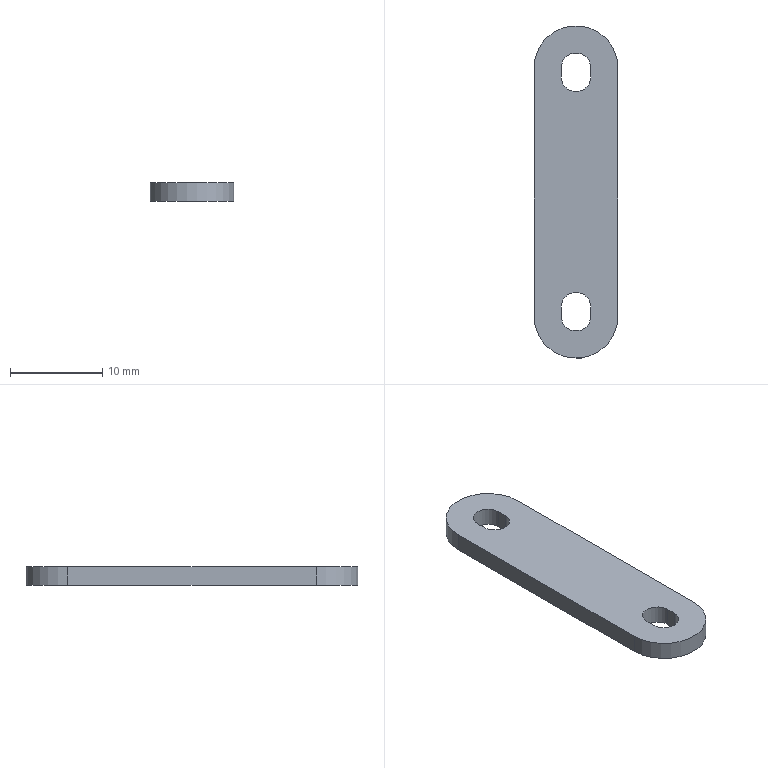Part | NX | features BREP 1 | 1 solid | 14 faces | box 9.123 x 36.123 x 2 mm | volume 578.449 mm3 | plane 8 | cylinder 6 | commonest cylinder face diameters 3.2 x4 9.123 x2
STEP:
#1=CARTESIAN_POINT('',(458.854,42.598,2.));
#2=VERTEX_POINT('',#1);
#3=CARTESIAN_POINT('',(449.731,42.598,2.));
#4=VERTEX_POINT('',#3);
#5=CARTESIAN_POINT('',(454.292,42.598,2.));
#6=DIRECTION('',(0.,0.,1.));
#7=DIRECTION('',(1.,0.,0.));
#8=AXIS2_PLACEMENT_3D('',#5,#6,#7);
#9=CIRCLE('',#8,4.562);
#10=EDGE_CURVE('',#2,#4,#9,.T.);
#11=ORIENTED_EDGE('',*,*,#10,.T.);
#12=CARTESIAN_POINT('',(449.731,15.598,2.));
#13=VERTEX_POINT('',#12);
#14=CARTESIAN_POINT('',(449.731,42.598,2.));
#15=DIRECTION('',(0.,-1.,0.));
#16=VECTOR('',#15,1000.);
#17=LINE('',#14,#16);
#18=EDGE_CURVE('',#4,#13,#17,.T.);
#19=ORIENTED_EDGE('',*,*,#18,.T.);
#20=CARTESIAN_POINT('',(458.854,15.598,2.));
#21=VERTEX_POINT('',#20);
#22=CARTESIAN_POINT('',(454.292,15.598,2.));
#23=DIRECTION('',(0.,0.,1.));
#24=DIRECTION('',(1.,0.,0.));
#25=AXIS2_PLACEMENT_3D('',#22,#23,#24);
#26=CIRCLE('',#25,4.562);
#27=EDGE_CURVE('',#13,#21,#26,.T.);
#28=ORIENTED_EDGE('',*,*,#27,.T.);
#29=CARTESIAN_POINT('',(458.854,42.598,2.));
#30=DIRECTION('',(0.,1.,0.));
#31=VECTOR('',#30,1000.);
#32=LINE('',#29,#31);
#33=EDGE_CURVE('',#21,#2,#32,.T.);
#34=ORIENTED_EDGE('',*,*,#33,.T.);
#35=EDGE_LOOP('',(#11,#19,#28,#34));
#36=FACE_BOUND('',#35,.T.);
#37=CARTESIAN_POINT('',(455.892,41.598,2.));
#38=VERTEX_POINT('',#37);
#39=CARTESIAN_POINT('',(455.892,42.598,2.));
#40=VERTEX_POINT('',#39);
#41=CARTESIAN_POINT('',(455.892,42.598,2.));
#42=DIRECTION('',(0.,1.,0.));
#43=VECTOR('',#42,1000.);
#44=LINE('',#41,#43);
#45=EDGE_CURVE('',#38,#40,#44,.T.);
#46=ORIENTED_EDGE('',*,*,#45,.F.);
#47=CARTESIAN_POINT('',(452.692,41.598,2.));
#48=VERTEX_POINT('',#47);
#49=CARTESIAN_POINT('',(454.292,41.598,2.));
#50=DIRECTION('',(0.,0.,1.));
#51=DIRECTION('',(1.,0.,0.));
#52=AXIS2_PLACEMENT_3D('',#49,#50,#51);
#53=CIRCLE('',#52,1.6);
#54=EDGE_CURVE('',#48,#38,#53,.T.);
#55=ORIENTED_EDGE('',*,*,#54,.F.);
#56=CARTESIAN_POINT('',(452.692,42.598,2.));
#57=VERTEX_POINT('',#56);
#58=CARTESIAN_POINT('',(452.692,42.598,2.));
#59=DIRECTION('',(0.,-1.,0.));
#60=VECTOR('',#59,1000.);
#61=LINE('',#58,#60);
#62=EDGE_CURVE('',#57,#48,#61,.T.);
#63=ORIENTED_EDGE('',*,*,#62,.F.);
#64=CARTESIAN_POINT('',(454.292,42.598,2.));
#65=DIRECTION('',(0.,0.,1.));
#66=DIRECTION('',(1.,0.,0.));
#67=AXIS2_PLACEMENT_3D('',#64,#65,#66);
#68=CIRCLE('',#67,1.6);
#69=EDGE_CURVE('',#40,#57,#68,.T.);
#70=ORIENTED_EDGE('',*,*,#69,.F.);
#71=EDGE_LOOP('',(#46,#55,#63,#70));
#72=FACE_BOUND('',#71,.T.);
#73=CARTESIAN_POINT('',(452.692,15.598,2.));
#74=VERTEX_POINT('',#73);
#75=CARTESIAN_POINT('',(455.892,15.598,2.));
#76=VERTEX_POINT('',#75);
#77=CARTESIAN_POINT('',(454.292,15.598,2.));
#78=DIRECTION('',(0.,0.,1.));
#79=DIRECTION('',(-1.,0.,0.));
#80=AXIS2_PLACEMENT_3D('',#77,#78,#79);
#81=CIRCLE('',#80,1.6);
#82=EDGE_CURVE('',#74,#76,#81,.T.);
#83=ORIENTED_EDGE('',*,*,#82,.F.);
#84=CARTESIAN_POINT('',(452.692,16.598,2.));
#85=VERTEX_POINT('',#84);
#86=CARTESIAN_POINT('',(452.692,15.598,2.));
#87=DIRECTION('',(0.,-1.,0.));
#88=VECTOR('',#87,1000.);
#89=LINE('',#86,#88);
#90=EDGE_CURVE('',#85,#74,#89,.T.);
#91=ORIENTED_EDGE('',*,*,#90,.F.);
#92=CARTESIAN_POINT('',(455.892,16.598,2.));
#93=VERTEX_POINT('',#92);
#94=CARTESIAN_POINT('',(454.292,16.598,2.));
#95=DIRECTION('',(0.,0.,1.));
#96=DIRECTION('',(-1.,0.,0.));
#97=AXIS2_PLACEMENT_3D('',#94,#95,#96);
#98=CIRCLE('',#97,1.6);
#99=EDGE_CURVE('',#93,#85,#98,.T.);
#100=ORIENTED_EDGE('',*,*,#99,.F.);
#101=CARTESIAN_POINT('',(455.892,15.598,2.));
#102=DIRECTION('',(0.,1.,0.));
#103=VECTOR('',#102,1000.);
#104=LINE('',#101,#103);
#105=EDGE_CURVE('',#76,#93,#104,.T.);
#106=ORIENTED_EDGE('',*,*,#105,.F.);
#107=EDGE_LOOP('',(#83,#91,#100,#106));
#108=FACE_BOUND('',#107,.T.);
#109=CARTESIAN_POINT('',(454.292,42.598,2.));
#110=DIRECTION('',(0.,0.,1.));
#111=DIRECTION('',(-1.,0.,0.));
#112=AXIS2_PLACEMENT_3D('',#109,#110,#111);
#113=PLANE('',#112);
#114=ADVANCED_FACE('',(#36,#72,#108),#113,.T.);
#115=CARTESIAN_POINT('',(458.854,42.598,0.));
#116=VERTEX_POINT('',#115);
#117=CARTESIAN_POINT('',(449.731,42.598,0.));
#118=VERTEX_POINT('',#117);
#119=CARTESIAN_POINT('',(454.292,42.598,0.));
#120=DIRECTION('',(0.,0.,1.));
#121=DIRECTION('',(1.,0.,0.));
#122=AXIS2_PLACEMENT_3D('',#119,#120,#121);
#123=CIRCLE('',#122,4.562);
#124=EDGE_CURVE('',#116,#118,#123,.T.);
#125=ORIENTED_EDGE('',*,*,#124,.F.);
#126=CARTESIAN_POINT('',(458.854,15.598,0.));
#127=VERTEX_POINT('',#126);
#128=CARTESIAN_POINT('',(458.854,42.598,0.));
#129=DIRECTION('',(0.,1.,0.));
#130=VECTOR('',#129,1000.);
#131=LINE('',#128,#130);
#132=EDGE_CURVE('',#127,#116,#131,.T.);
#133=ORIENTED_EDGE('',*,*,#132,.F.);
#134=CARTESIAN_POINT('',(449.731,15.598,0.));
#135=VERTEX_POINT('',#134);
#136=CARTESIAN_POINT('',(454.292,15.598,0.));
#137=DIRECTION('',(0.,0.,1.));
#138=DIRECTION('',(1.,0.,0.));
#139=AXIS2_PLACEMENT_3D('',#136,#137,#138);
#140=CIRCLE('',#139,4.562);
#141=EDGE_CURVE('',#135,#127,#140,.T.);
#142=ORIENTED_EDGE('',*,*,#141,.F.);
#143=CARTESIAN_POINT('',(449.731,42.598,0.));
#144=DIRECTION('',(0.,-1.,0.));
#145=VECTOR('',#144,1000.);
#146=LINE('',#143,#145);
#147=EDGE_CURVE('',#118,#135,#146,.T.);
#148=ORIENTED_EDGE('',*,*,#147,.F.);
#149=EDGE_LOOP('',(#125,#133,#142,#148));
#150=FACE_BOUND('',#149,.T.);
#151=CARTESIAN_POINT('',(452.692,16.598,0.));
#152=VERTEX_POINT('',#151);
#153=CARTESIAN_POINT('',(452.692,15.598,0.));
#154=VERTEX_POINT('',#153);
#155=CARTESIAN_POINT('',(452.692,42.598,0.));
#156=DIRECTION('',(0.,-1.,0.));
#157=VECTOR('',#156,1000.);
#158=LINE('',#155,#157);
#159=EDGE_CURVE('',#152,#154,#158,.T.);
#160=ORIENTED_EDGE('',*,*,#159,.T.);
#161=CARTESIAN_POINT('',(455.892,15.598,0.));
#162=VERTEX_POINT('',#161);
#163=CARTESIAN_POINT('',(454.292,15.598,0.));
#164=DIRECTION('',(0.,0.,1.));
#165=DIRECTION('',(1.,0.,0.));
#166=AXIS2_PLACEMENT_3D('',#163,#164,#165);
#167=CIRCLE('',#166,1.6);
#168=EDGE_CURVE('',#154,#162,#167,.T.);
#169=ORIENTED_EDGE('',*,*,#168,.T.);
#170=CARTESIAN_POINT('',(455.892,16.598,0.));
#171=VERTEX_POINT('',#170);
#172=CARTESIAN_POINT('',(455.892,42.598,0.));
#173=DIRECTION('',(0.,1.,0.));
#174=VECTOR('',#173,1000.);
#175=LINE('',#172,#174);
#176=EDGE_CURVE('',#162,#171,#175,.T.);
#177=ORIENTED_EDGE('',*,*,#176,.T.);
#178=CARTESIAN_POINT('',(454.292,16.598,0.));
#179=DIRECTION('',(0.,0.,1.));
#180=DIRECTION('',(1.,0.,0.));
#181=AXIS2_PLACEMENT_3D('',#178,#179,#180);
#182=CIRCLE('',#181,1.6);
#183=EDGE_CURVE('',#171,#152,#182,.T.);
#184=ORIENTED_EDGE('',*,*,#183,.T.);
#185=EDGE_LOOP('',(#160,#169,#177,#184));
#186=FACE_BOUND('',#185,.T.);
#187=CARTESIAN_POINT('',(452.692,41.598,0.));
#188=VERTEX_POINT('',#187);
#189=CARTESIAN_POINT('',(455.892,41.598,0.));
#190=VERTEX_POINT('',#189);
#191=CARTESIAN_POINT('',(454.292,41.598,0.));
#192=DIRECTION('',(0.,0.,1.));
#193=DIRECTION('',(1.,0.,0.));
#194=AXIS2_PLACEMENT_3D('',#191,#192,#193);
#195=CIRCLE('',#194,1.6);
#196=EDGE_CURVE('',#188,#190,#195,.T.);
#197=ORIENTED_EDGE('',*,*,#196,.T.);
#198=CARTESIAN_POINT('',(455.892,42.598,0.));
#199=VERTEX_POINT('',#198);
#200=CARTESIAN_POINT('',(455.892,42.598,0.));
#201=DIRECTION('',(0.,1.,0.));
#202=VECTOR('',#201,1000.);
#203=LINE('',#200,#202);
#204=EDGE_CURVE('',#190,#199,#203,.T.);
#205=ORIENTED_EDGE('',*,*,#204,.T.);
#206=CARTESIAN_POINT('',(452.692,42.598,0.));
#207=VERTEX_POINT('',#206);
#208=CARTESIAN_POINT('',(454.292,42.598,0.));
#209=DIRECTION('',(0.,0.,1.));
#210=DIRECTION('',(1.,0.,0.));
#211=AXIS2_PLACEMENT_3D('',#208,#209,#210);
#212=CIRCLE('',#211,1.6);
#213=EDGE_CURVE('',#199,#207,#212,.T.);
#214=ORIENTED_EDGE('',*,*,#213,.T.);
#215=CARTESIAN_POINT('',(452.692,42.598,0.));
#216=DIRECTION('',(0.,-1.,0.));
#217=VECTOR('',#216,1000.);
#218=LINE('',#215,#217);
#219=EDGE_CURVE('',#207,#188,#218,.T.);
#220=ORIENTED_EDGE('',*,*,#219,.T.);
#221=EDGE_LOOP('',(#197,#205,#214,#220));
#222=FACE_BOUND('',#221,.T.);
#223=CARTESIAN_POINT('',(454.292,42.598,0.));
#224=DIRECTION('',(0.,0.,1.));
#225=DIRECTION('',(-1.,0.,0.));
#226=AXIS2_PLACEMENT_3D('',#223,#224,#225);
#227=PLANE('',#226);
#228=ADVANCED_FACE('',(#150,#186,#222),#227,.F.);
#229=ORIENTED_EDGE('',*,*,#124,.T.);
#230=CARTESIAN_POINT('',(449.731,42.598,2.));
#231=DIRECTION('',(0.,0.,-1.));
#232=VECTOR('',#231,1000.);
#233=LINE('',#230,#232);
#234=EDGE_CURVE('',#4,#118,#233,.T.);
#235=ORIENTED_EDGE('',*,*,#234,.F.);
#236=ORIENTED_EDGE('',*,*,#10,.F.);
#237=CARTESIAN_POINT('',(458.854,42.598,2.));
#238=DIRECTION('',(0.,0.,-1.));
#239=VECTOR('',#238,1000.);
#240=LINE('',#237,#239);
#241=EDGE_CURVE('',#2,#116,#240,.T.);
#242=ORIENTED_EDGE('',*,*,#241,.T.);
#243=EDGE_LOOP('',(#229,#235,#236,#242));
#244=FACE_BOUND('',#243,.T.);
#245=CARTESIAN_POINT('',(454.292,42.598,2.));
#246=DIRECTION('',(0.,0.,-1.));
#247=DIRECTION('',(1.,0.,0.));
#248=AXIS2_PLACEMENT_3D('',#245,#246,#247);
#249=CYLINDRICAL_SURFACE('',#248,4.562);
#250=ADVANCED_FACE('',(#244),#249,.T.);
#251=ORIENTED_EDGE('',*,*,#147,.T.);
#252=CARTESIAN_POINT('',(449.731,15.598,2.));
#253=DIRECTION('',(0.,0.,-1.));
#254=VECTOR('',#253,1000.);
#255=LINE('',#252,#254);
#256=EDGE_CURVE('',#13,#135,#255,.T.);
#257=ORIENTED_EDGE('',*,*,#256,.F.);
#258=ORIENTED_EDGE('',*,*,#18,.F.);
#259=ORIENTED_EDGE('',*,*,#234,.T.);
#260=EDGE_LOOP('',(#251,#257,#258,#259));
#261=FACE_BOUND('',#260,.T.);
#262=CARTESIAN_POINT('',(449.731,42.598,2.));
#263=DIRECTION('',(1.,0.,0.));
#264=DIRECTION('',(0.,-1.,0.));
#265=AXIS2_PLACEMENT_3D('',#262,#263,#264);
#266=PLANE('',#265);
#267=ADVANCED_FACE('',(#261),#266,.F.);
#268=ORIENTED_EDGE('',*,*,#141,.T.);
#269=CARTESIAN_POINT('',(458.854,15.598,2.));
#270=DIRECTION('',(0.,0.,-1.));
#271=VECTOR('',#270,1000.);
#272=LINE('',#269,#271);
#273=EDGE_CURVE('',#21,#127,#272,.T.);
#274=ORIENTED_EDGE('',*,*,#273,.F.);
#275=ORIENTED_EDGE('',*,*,#27,.F.);
#276=ORIENTED_EDGE('',*,*,#256,.T.);
#277=EDGE_LOOP('',(#268,#274,#275,#276));
#278=FACE_BOUND('',#277,.T.);
#279=CARTESIAN_POINT('',(454.292,15.598,2.));
#280=DIRECTION('',(0.,0.,-1.));
#281=DIRECTION('',(1.,0.,0.));
#282=AXIS2_PLACEMENT_3D('',#279,#280,#281);
#283=CYLINDRICAL_SURFACE('',#282,4.562);
#284=ADVANCED_FACE('',(#278),#283,.T.);
#285=ORIENTED_EDGE('',*,*,#132,.T.);
#286=ORIENTED_EDGE('',*,*,#241,.F.);
#287=ORIENTED_EDGE('',*,*,#33,.F.);
#288=ORIENTED_EDGE('',*,*,#273,.T.);
#289=EDGE_LOOP('',(#285,#286,#287,#288));
#290=FACE_BOUND('',#289,.T.);
#291=CARTESIAN_POINT('',(458.854,42.598,2.));
#292=DIRECTION('',(-1.,0.,0.));
#293=DIRECTION('',(0.,0.,-1.));
#294=AXIS2_PLACEMENT_3D('',#291,#292,#293);
#295=PLANE('',#294);
#296=ADVANCED_FACE('',(#290),#295,.F.);
#297=CARTESIAN_POINT('',(455.892,42.598,2.));
#298=DIRECTION('',(0.,0.,-1.));
#299=VECTOR('',#298,1000.);
#300=LINE('',#297,#299);
#301=EDGE_CURVE('',#40,#199,#300,.T.);
#302=ORIENTED_EDGE('',*,*,#301,.F.);
#303=ORIENTED_EDGE('',*,*,#69,.T.);
#304=CARTESIAN_POINT('',(452.692,42.598,2.));
#305=DIRECTION('',(0.,0.,-1.));
#306=VECTOR('',#305,1000.);
#307=LINE('',#304,#306);
#308=EDGE_CURVE('',#57,#207,#307,.T.);
#309=ORIENTED_EDGE('',*,*,#308,.T.);
#310=ORIENTED_EDGE('',*,*,#213,.F.);
#311=EDGE_LOOP('',(#302,#303,#309,#310));
#312=FACE_BOUND('',#311,.T.);
#313=CARTESIAN_POINT('',(454.292,42.598,2.));
#314=DIRECTION('',(0.,0.,-1.));
#315=DIRECTION('',(1.,0.,0.));
#316=AXIS2_PLACEMENT_3D('',#313,#314,#315);
#317=CYLINDRICAL_SURFACE('',#316,1.6);
#318=ADVANCED_FACE('',(#312),#317,.F.);
#319=CARTESIAN_POINT('',(452.692,41.598,-8.));
#320=DIRECTION('',(0.,0.,1.));
#321=VECTOR('',#320,1000.);
#322=LINE('',#319,#321);
#323=EDGE_CURVE('',#188,#48,#322,.T.);
#324=ORIENTED_EDGE('',*,*,#323,.T.);
#325=ORIENTED_EDGE('',*,*,#54,.T.);
#326=CARTESIAN_POINT('',(455.892,41.598,-8.));
#327=DIRECTION('',(0.,0.,1.));
#328=VECTOR('',#327,1000.);
#329=LINE('',#326,#328);
#330=EDGE_CURVE('',#190,#38,#329,.T.);
#331=ORIENTED_EDGE('',*,*,#330,.F.);
#332=ORIENTED_EDGE('',*,*,#196,.F.);
#333=EDGE_LOOP('',(#324,#325,#331,#332));
#334=FACE_BOUND('',#333,.T.);
#335=CARTESIAN_POINT('',(454.292,41.598,-8.));
#336=DIRECTION('',(0.,0.,1.));
#337=DIRECTION('',(-1.,0.,0.));
#338=AXIS2_PLACEMENT_3D('',#335,#336,#337);
#339=CYLINDRICAL_SURFACE('',#338,1.6);
#340=ADVANCED_FACE('',(#334),#339,.F.);
#341=ORIENTED_EDGE('',*,*,#330,.T.);
#342=ORIENTED_EDGE('',*,*,#45,.T.);
#343=ORIENTED_EDGE('',*,*,#301,.T.);
#344=ORIENTED_EDGE('',*,*,#204,.F.);
#345=EDGE_LOOP('',(#341,#342,#343,#344));
#346=FACE_BOUND('',#345,.T.);
#347=CARTESIAN_POINT('',(455.892,42.598,-8.));
#348=DIRECTION('',(1.,0.,0.));
#349=DIRECTION('',(0.,-1.,0.));
#350=AXIS2_PLACEMENT_3D('',#347,#348,#349);
#351=PLANE('',#350);
#352=ADVANCED_FACE('',(#346),#351,.F.);
#353=ORIENTED_EDGE('',*,*,#308,.F.);
#354=ORIENTED_EDGE('',*,*,#62,.T.);
#355=ORIENTED_EDGE('',*,*,#323,.F.);
#356=ORIENTED_EDGE('',*,*,#219,.F.);
#357=EDGE_LOOP('',(#353,#354,#355,#356));
#358=FACE_BOUND('',#357,.T.);
#359=CARTESIAN_POINT('',(452.692,42.598,-8.));
#360=DIRECTION('',(-1.,0.,0.));
#361=DIRECTION('',(0.,0.,-1.));
#362=AXIS2_PLACEMENT_3D('',#359,#360,#361);
#363=PLANE('',#362);
#364=ADVANCED_FACE('',(#358),#363,.F.);
#365=CARTESIAN_POINT('',(452.692,15.598,-8.));
#366=DIRECTION('',(0.,0.,1.));
#367=VECTOR('',#366,1000.);
#368=LINE('',#365,#367);
#369=EDGE_CURVE('',#154,#74,#368,.T.);
#370=ORIENTED_EDGE('',*,*,#369,.T.);
#371=ORIENTED_EDGE('',*,*,#82,.T.);
#372=CARTESIAN_POINT('',(455.892,15.598,-8.));
#373=DIRECTION('',(0.,0.,1.));
#374=VECTOR('',#373,1000.);
#375=LINE('',#372,#374);
#376=EDGE_CURVE('',#162,#76,#375,.T.);
#377=ORIENTED_EDGE('',*,*,#376,.F.);
#378=ORIENTED_EDGE('',*,*,#168,.F.);
#379=EDGE_LOOP('',(#370,#371,#377,#378));
#380=FACE_BOUND('',#379,.T.);
#381=CARTESIAN_POINT('',(454.292,15.598,-8.));
#382=DIRECTION('',(0.,0.,1.));
#383=DIRECTION('',(-1.,0.,0.));
#384=AXIS2_PLACEMENT_3D('',#381,#382,#383);
#385=CYLINDRICAL_SURFACE('',#384,1.6);
#386=ADVANCED_FACE('',(#380),#385,.F.);
#387=CARTESIAN_POINT('',(452.692,16.598,-8.));
#388=DIRECTION('',(0.,0.,1.));
#389=VECTOR('',#388,1000.);
#390=LINE('',#387,#389);
#391=EDGE_CURVE('',#152,#85,#390,.T.);
#392=ORIENTED_EDGE('',*,*,#391,.T.);
#393=ORIENTED_EDGE('',*,*,#90,.T.);
#394=ORIENTED_EDGE('',*,*,#369,.F.);
#395=ORIENTED_EDGE('',*,*,#159,.F.);
#396=EDGE_LOOP('',(#392,#393,#394,#395));
#397=FACE_BOUND('',#396,.T.);
#398=CARTESIAN_POINT('',(452.692,15.598,-8.));
#399=DIRECTION('',(-1.,0.,0.));
#400=DIRECTION('',(0.,0.,-1.));
#401=AXIS2_PLACEMENT_3D('',#398,#399,#400);
#402=PLANE('',#401);
#403=ADVANCED_FACE('',(#397),#402,.F.);
#404=CARTESIAN_POINT('',(455.892,16.598,-8.));
#405=DIRECTION('',(0.,0.,1.));
#406=VECTOR('',#405,1000.);
#407=LINE('',#404,#406);
#408=EDGE_CURVE('',#171,#93,#407,.T.);
#409=ORIENTED_EDGE('',*,*,#408,.T.);
#410=ORIENTED_EDGE('',*,*,#99,.T.);
#411=ORIENTED_EDGE('',*,*,#391,.F.);
#412=ORIENTED_EDGE('',*,*,#183,.F.);
#413=EDGE_LOOP('',(#409,#410,#411,#412));
#414=FACE_BOUND('',#413,.T.);
#415=CARTESIAN_POINT('',(454.292,16.598,-8.));
#416=DIRECTION('',(0.,0.,1.));
#417=DIRECTION('',(-1.,0.,0.));
#418=AXIS2_PLACEMENT_3D('',#415,#416,#417);
#419=CYLINDRICAL_SURFACE('',#418,1.6);
#420=ADVANCED_FACE('',(#414),#419,.F.);
#421=ORIENTED_EDGE('',*,*,#376,.T.);
#422=ORIENTED_EDGE('',*,*,#105,.T.);
#423=ORIENTED_EDGE('',*,*,#408,.F.);
#424=ORIENTED_EDGE('',*,*,#176,.F.);
#425=EDGE_LOOP('',(#421,#422,#423,#424));
#426=FACE_BOUND('',#425,.T.);
#427=CARTESIAN_POINT('',(455.892,15.598,-8.));
#428=DIRECTION('',(1.,0.,0.));
#429=DIRECTION('',(0.,-1.,0.));
#430=AXIS2_PLACEMENT_3D('',#427,#428,#429);
#431=PLANE('',#430);
#432=ADVANCED_FACE('',(#426),#431,.F.);
#433=CLOSED_SHELL('',(#114,#228,#250,#267,#284,#296,#318,#340,#352,#364,#386,#403,#420,#432));
#434=MANIFOLD_SOLID_BREP('',#433);
#435=(LENGTH_UNIT()NAMED_UNIT(*)SI_UNIT(.MILLI.,.METRE.));
#436=UNCERTAINTY_MEASURE_WITH_UNIT(LENGTH_MEASURE(0.00001),#435,'','');
#437=(NAMED_UNIT(*)PLANE_ANGLE_UNIT()SI_UNIT($,.RADIAN.));
#438=(NAMED_UNIT(*)SI_UNIT($,.STERADIAN.)SOLID_ANGLE_UNIT());
#439=(GEOMETRIC_REPRESENTATION_CONTEXT(3)GLOBAL_UNCERTAINTY_ASSIGNED_CONTEXT((#436))GLOBAL_UNIT_ASSIGNED_CONTEXT((#435,#437,#438))REPRESENTATION_CONTEXT('',''));
#440=ADVANCED_BREP_SHAPE_REPRESENTATION('',(#434),#439);